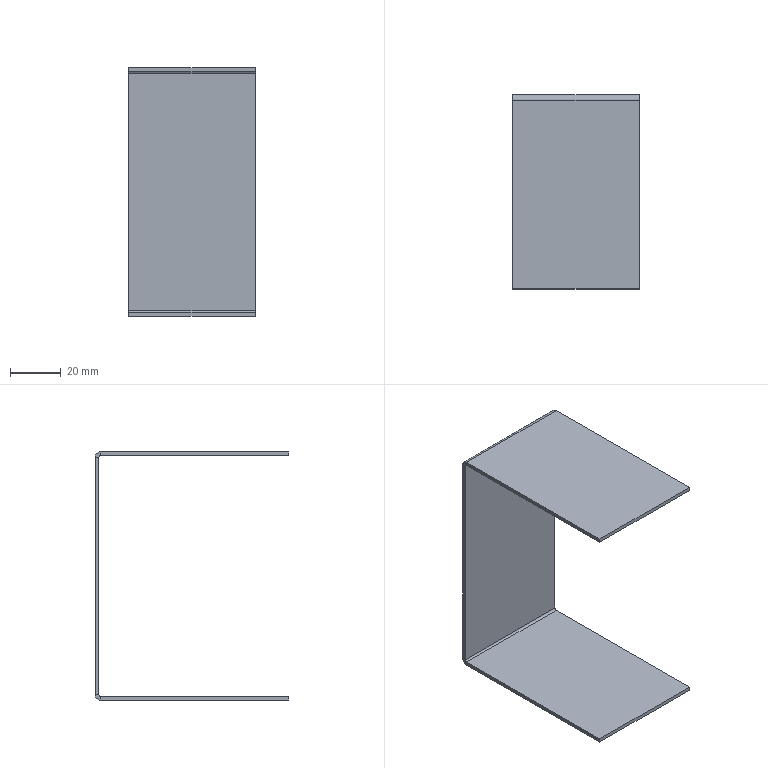Part | NX | 1 solid | 22 faces | box 50 x 76.5 x 98 mm | volume 18504 mm3 | plane 18 | cylinder 4 | commonest cylinder face diameters 1.473 x2 4.473 x2
STEP:
#1=CARTESIAN_POINT('',(-25.,-1.5,-46.763));
#2=VERTEX_POINT('',#1);
#3=CARTESIAN_POINT('',(-25.,-1.5,46.763));
#4=VERTEX_POINT('',#3);
#5=CARTESIAN_POINT('',(-25.,-1.5,47.5));
#6=DIRECTION('',(0.,0.,1.));
#7=VECTOR('',#6,1000.);
#8=LINE('',#5,#7);
#9=EDGE_CURVE('',#2,#4,#8,.T.);
#10=ORIENTED_EDGE('',*,*,#9,.F.);
#11=CARTESIAN_POINT('',(25.,-1.5,-46.763));
#12=VERTEX_POINT('',#11);
#13=CARTESIAN_POINT('',(25.,-1.5,-46.763));
#14=DIRECTION('',(1.,0.,0.));
#15=VECTOR('',#14,1000.);
#16=LINE('',#13,#15);
#17=EDGE_CURVE('',#12,#2,#16,.F.);
#18=ORIENTED_EDGE('',*,*,#17,.F.);
#19=CARTESIAN_POINT('',(25.,-1.5,46.763));
#20=VERTEX_POINT('',#19);
#21=CARTESIAN_POINT('',(25.,-1.5,47.5));
#22=DIRECTION('',(0.,0.,-1.));
#23=VECTOR('',#22,1000.);
#24=LINE('',#21,#23);
#25=EDGE_CURVE('',#20,#12,#24,.T.);
#26=ORIENTED_EDGE('',*,*,#25,.F.);
#27=CARTESIAN_POINT('',(-25.,-1.5,46.763));
#28=DIRECTION('',(-1.,0.,0.));
#29=VECTOR('',#28,1000.);
#30=LINE('',#27,#29);
#31=EDGE_CURVE('',#4,#20,#30,.F.);
#32=ORIENTED_EDGE('',*,*,#31,.F.);
#33=EDGE_LOOP('',(#10,#18,#26,#32));
#34=FACE_BOUND('',#33,.T.);
#35=CARTESIAN_POINT('',(0.,-1.5,0.));
#36=DIRECTION('',(0.,-1.,0.));
#37=DIRECTION('',(0.,0.,-1.));
#38=AXIS2_PLACEMENT_3D('',#35,#36,#37);
#39=PLANE('',#38);
#40=ADVANCED_FACE('',(#34),#39,.T.);
#41=CARTESIAN_POINT('',(25.,0.,-46.763));
#42=VERTEX_POINT('',#41);
#43=CARTESIAN_POINT('',(-25.,0.,-46.763));
#44=VERTEX_POINT('',#43);
#45=CARTESIAN_POINT('',(25.,0.,-46.763));
#46=DIRECTION('',(1.,0.,0.));
#47=VECTOR('',#46,1000.);
#48=LINE('',#45,#47);
#49=EDGE_CURVE('',#42,#44,#48,.F.);
#50=ORIENTED_EDGE('',*,*,#49,.T.);
#51=CARTESIAN_POINT('',(-25.,0.,46.763));
#52=VERTEX_POINT('',#51);
#53=CARTESIAN_POINT('',(-25.,0.,47.5));
#54=DIRECTION('',(0.,0.,1.));
#55=VECTOR('',#54,1000.);
#56=LINE('',#53,#55);
#57=EDGE_CURVE('',#44,#52,#56,.T.);
#58=ORIENTED_EDGE('',*,*,#57,.T.);
#59=CARTESIAN_POINT('',(25.,0.,46.763));
#60=VERTEX_POINT('',#59);
#61=CARTESIAN_POINT('',(-25.,0.,46.763));
#62=DIRECTION('',(-1.,0.,0.));
#63=VECTOR('',#62,1000.);
#64=LINE('',#61,#63);
#65=EDGE_CURVE('',#52,#60,#64,.F.);
#66=ORIENTED_EDGE('',*,*,#65,.T.);
#67=CARTESIAN_POINT('',(25.,0.,47.5));
#68=DIRECTION('',(0.,0.,-1.));
#69=VECTOR('',#68,1000.);
#70=LINE('',#67,#69);
#71=EDGE_CURVE('',#60,#42,#70,.T.);
#72=ORIENTED_EDGE('',*,*,#71,.T.);
#73=EDGE_LOOP('',(#50,#58,#66,#72));
#74=FACE_BOUND('',#73,.T.);
#75=CARTESIAN_POINT('',(0.,0.,0.));
#76=DIRECTION('',(0.,-1.,0.));
#77=DIRECTION('',(0.,0.,-1.));
#78=AXIS2_PLACEMENT_3D('',#75,#76,#77);
#79=PLANE('',#78);
#80=ADVANCED_FACE('',(#74),#79,.F.);
#81=ORIENTED_EDGE('',*,*,#25,.T.);
#82=CARTESIAN_POINT('',(25.,-1.5,-46.763));
#83=DIRECTION('',(0.,1.,0.));
#84=VECTOR('',#83,1000.);
#85=LINE('',#82,#84);
#86=EDGE_CURVE('',#12,#42,#85,.T.);
#87=ORIENTED_EDGE('',*,*,#86,.T.);
#88=ORIENTED_EDGE('',*,*,#71,.F.);
#89=CARTESIAN_POINT('',(25.,-1.5,46.763));
#90=DIRECTION('',(0.,1.,0.));
#91=VECTOR('',#90,1000.);
#92=LINE('',#89,#91);
#93=EDGE_CURVE('',#20,#60,#92,.T.);
#94=ORIENTED_EDGE('',*,*,#93,.F.);
#95=EDGE_LOOP('',(#81,#87,#88,#94));
#96=FACE_BOUND('',#95,.T.);
#97=CARTESIAN_POINT('',(25.,-1.5,47.5));
#98=DIRECTION('',(1.,0.,0.));
#99=DIRECTION('',(0.,0.,-1.));
#100=AXIS2_PLACEMENT_3D('',#97,#98,#99);
#101=PLANE('',#100);
#102=ADVANCED_FACE('',(#96),#101,.T.);
#103=CARTESIAN_POINT('',(-25.,-1.5,-46.763));
#104=DIRECTION('',(0.,1.,0.));
#105=VECTOR('',#104,1000.);
#106=LINE('',#103,#105);
#107=EDGE_CURVE('',#2,#44,#106,.T.);
#108=ORIENTED_EDGE('',*,*,#107,.F.);
#109=ORIENTED_EDGE('',*,*,#9,.T.);
#110=CARTESIAN_POINT('',(-25.,-1.5,46.763));
#111=DIRECTION('',(0.,1.,0.));
#112=VECTOR('',#111,1000.);
#113=LINE('',#110,#112);
#114=EDGE_CURVE('',#4,#52,#113,.T.);
#115=ORIENTED_EDGE('',*,*,#114,.T.);
#116=ORIENTED_EDGE('',*,*,#57,.F.);
#117=EDGE_LOOP('',(#108,#109,#115,#116));
#118=FACE_BOUND('',#117,.T.);
#119=CARTESIAN_POINT('',(-25.,-1.5,47.5));
#120=DIRECTION('',(-1.,0.,0.));
#121=DIRECTION('',(0.,0.,1.));
#122=AXIS2_PLACEMENT_3D('',#119,#120,#121);
#123=PLANE('',#122);
#124=ADVANCED_FACE('',(#118),#123,.T.);
#125=CARTESIAN_POINT('',(25.,-2.237,47.5));
#126=VERTEX_POINT('',#125);
#127=CARTESIAN_POINT('',(25.,-2.237,49.));
#128=VERTEX_POINT('',#127);
#129=CARTESIAN_POINT('',(25.,-2.237,47.5));
#130=DIRECTION('',(0.,0.,1.));
#131=VECTOR('',#130,1000.);
#132=LINE('',#129,#131);
#133=EDGE_CURVE('',#126,#128,#132,.T.);
#134=ORIENTED_EDGE('',*,*,#133,.F.);
#135=CARTESIAN_POINT('',(25.,-2.237,46.763));
#136=DIRECTION('',(-1.,0.,0.));
#137=DIRECTION('',(0.,0.,1.));
#138=AXIS2_PLACEMENT_3D('',#135,#136,#137);
#139=CIRCLE('',#138,0.7366);
#140=EDGE_CURVE('',#20,#126,#139,.F.);
#141=ORIENTED_EDGE('',*,*,#140,.F.);
#142=ORIENTED_EDGE('',*,*,#93,.T.);
#143=CARTESIAN_POINT('',(25.,-2.237,46.763));
#144=DIRECTION('',(-1.,0.,0.));
#145=DIRECTION('',(0.,0.,1.));
#146=AXIS2_PLACEMENT_3D('',#143,#144,#145);
#147=CIRCLE('',#146,2.237);
#148=EDGE_CURVE('',#60,#128,#147,.F.);
#149=ORIENTED_EDGE('',*,*,#148,.T.);
#150=EDGE_LOOP('',(#134,#141,#142,#149));
#151=FACE_BOUND('',#150,.T.);
#152=CARTESIAN_POINT('',(25.,-2.237,46.763));
#153=DIRECTION('',(1.,0.,0.));
#154=DIRECTION('',(0.,0.,-1.));
#155=AXIS2_PLACEMENT_3D('',#152,#153,#154);
#156=PLANE('',#155);
#157=ADVANCED_FACE('',(#151),#156,.T.);
#158=CARTESIAN_POINT('',(-25.,-2.237,47.5));
#159=VERTEX_POINT('',#158);
#160=CARTESIAN_POINT('',(-25.,-2.237,46.763));
#161=DIRECTION('',(-1.,0.,0.));
#162=DIRECTION('',(0.,0.,1.));
#163=AXIS2_PLACEMENT_3D('',#160,#161,#162);
#164=CIRCLE('',#163,0.7366);
#165=EDGE_CURVE('',#159,#4,#164,.T.);
#166=ORIENTED_EDGE('',*,*,#165,.F.);
#167=CARTESIAN_POINT('',(-25.,-2.237,49.));
#168=VERTEX_POINT('',#167);
#169=CARTESIAN_POINT('',(-25.,-2.237,47.5));
#170=DIRECTION('',(0.,0.,1.));
#171=VECTOR('',#170,1000.);
#172=LINE('',#169,#171);
#173=EDGE_CURVE('',#159,#168,#172,.T.);
#174=ORIENTED_EDGE('',*,*,#173,.T.);
#175=CARTESIAN_POINT('',(-25.,-2.237,46.763));
#176=DIRECTION('',(-1.,0.,0.));
#177=DIRECTION('',(0.,0.,1.));
#178=AXIS2_PLACEMENT_3D('',#175,#176,#177);
#179=CIRCLE('',#178,2.237);
#180=EDGE_CURVE('',#168,#52,#179,.T.);
#181=ORIENTED_EDGE('',*,*,#180,.T.);
#182=ORIENTED_EDGE('',*,*,#114,.F.);
#183=EDGE_LOOP('',(#166,#174,#181,#182));
#184=FACE_BOUND('',#183,.T.);
#185=CARTESIAN_POINT('',(-25.,-2.237,46.763));
#186=DIRECTION('',(1.,0.,0.));
#187=DIRECTION('',(0.,0.,-1.));
#188=AXIS2_PLACEMENT_3D('',#185,#186,#187);
#189=PLANE('',#188);
#190=ADVANCED_FACE('',(#184),#189,.F.);
#191=ORIENTED_EDGE('',*,*,#65,.F.);
#192=ORIENTED_EDGE('',*,*,#180,.F.);
#193=CARTESIAN_POINT('',(0.,-2.237,49.));
#194=DIRECTION('',(-1.,0.,0.));
#195=VECTOR('',#194,1000.);
#196=LINE('',#193,#195);
#197=EDGE_CURVE('',#128,#168,#196,.T.);
#198=ORIENTED_EDGE('',*,*,#197,.F.);
#199=ORIENTED_EDGE('',*,*,#148,.F.);
#200=EDGE_LOOP('',(#191,#192,#198,#199));
#201=FACE_BOUND('',#200,.T.);
#202=CARTESIAN_POINT('',(-25.,-2.237,46.763));
#203=DIRECTION('',(-1.,0.,0.));
#204=DIRECTION('',(0.,0.,1.));
#205=AXIS2_PLACEMENT_3D('',#202,#203,#204);
#206=CYLINDRICAL_SURFACE('',#205,2.237);
#207=ADVANCED_FACE('',(#201),#206,.T.);
#208=ORIENTED_EDGE('',*,*,#31,.T.);
#209=ORIENTED_EDGE('',*,*,#140,.T.);
#210=CARTESIAN_POINT('',(25.,-2.237,47.5));
#211=DIRECTION('',(-1.,0.,0.));
#212=VECTOR('',#211,1000.);
#213=LINE('',#210,#212);
#214=EDGE_CURVE('',#126,#159,#213,.T.);
#215=ORIENTED_EDGE('',*,*,#214,.T.);
#216=ORIENTED_EDGE('',*,*,#165,.T.);
#217=EDGE_LOOP('',(#208,#209,#215,#216));
#218=FACE_BOUND('',#217,.T.);
#219=CARTESIAN_POINT('',(-25.,-2.237,46.763));
#220=DIRECTION('',(-1.,0.,0.));
#221=DIRECTION('',(0.,0.,1.));
#222=AXIS2_PLACEMENT_3D('',#219,#220,#221);
#223=CYLINDRICAL_SURFACE('',#222,0.7366);
#224=ADVANCED_FACE('',(#218),#223,.F.);
#225=CARTESIAN_POINT('',(-25.,-76.5,49.));
#226=VERTEX_POINT('',#225);
#227=CARTESIAN_POINT('',(-25.,-1.5,49.));
#228=DIRECTION('',(0.,1.,0.));
#229=VECTOR('',#228,1000.);
#230=LINE('',#227,#229);
#231=EDGE_CURVE('',#226,#168,#230,.T.);
#232=ORIENTED_EDGE('',*,*,#231,.T.);
#233=ORIENTED_EDGE('',*,*,#173,.F.);
#234=CARTESIAN_POINT('',(-25.,-76.5,47.5));
#235=VERTEX_POINT('',#234);
#236=CARTESIAN_POINT('',(-25.,-1.5,47.5));
#237=DIRECTION('',(0.,1.,0.));
#238=VECTOR('',#237,1000.);
#239=LINE('',#236,#238);
#240=EDGE_CURVE('',#235,#159,#239,.T.);
#241=ORIENTED_EDGE('',*,*,#240,.F.);
#242=CARTESIAN_POINT('',(-25.,-76.5,49.));
#243=DIRECTION('',(0.,0.,-1.));
#244=VECTOR('',#243,1000.);
#245=LINE('',#242,#244);
#246=EDGE_CURVE('',#226,#235,#245,.T.);
#247=ORIENTED_EDGE('',*,*,#246,.F.);
#248=EDGE_LOOP('',(#232,#233,#241,#247));
#249=FACE_BOUND('',#248,.T.);
#250=CARTESIAN_POINT('',(-25.,-1.5,49.));
#251=DIRECTION('',(-1.,0.,0.));
#252=DIRECTION('',(0.,-1.,0.));
#253=AXIS2_PLACEMENT_3D('',#250,#251,#252);
#254=PLANE('',#253);
#255=ADVANCED_FACE('',(#249),#254,.T.);
#256=CARTESIAN_POINT('',(25.,-76.5,47.5));
#257=VERTEX_POINT('',#256);
#258=CARTESIAN_POINT('',(25.,-76.5,47.5));
#259=DIRECTION('',(0.,-1.,0.));
#260=VECTOR('',#259,1000.);
#261=LINE('',#258,#260);
#262=EDGE_CURVE('',#126,#257,#261,.T.);
#263=ORIENTED_EDGE('',*,*,#262,.F.);
#264=ORIENTED_EDGE('',*,*,#133,.T.);
#265=CARTESIAN_POINT('',(25.,-76.5,49.));
#266=VERTEX_POINT('',#265);
#267=CARTESIAN_POINT('',(25.,-76.5,49.));
#268=DIRECTION('',(0.,-1.,0.));
#269=VECTOR('',#268,1000.);
#270=LINE('',#267,#269);
#271=EDGE_CURVE('',#128,#266,#270,.T.);
#272=ORIENTED_EDGE('',*,*,#271,.T.);
#273=CARTESIAN_POINT('',(25.,-76.5,49.));
#274=DIRECTION('',(0.,0.,-1.));
#275=VECTOR('',#274,1000.);
#276=LINE('',#273,#275);
#277=EDGE_CURVE('',#266,#257,#276,.T.);
#278=ORIENTED_EDGE('',*,*,#277,.T.);
#279=EDGE_LOOP('',(#263,#264,#272,#278));
#280=FACE_BOUND('',#279,.T.);
#281=CARTESIAN_POINT('',(25.,-76.5,49.));
#282=DIRECTION('',(1.,0.,0.));
#283=DIRECTION('',(0.,1.,0.));
#284=AXIS2_PLACEMENT_3D('',#281,#282,#283);
#285=PLANE('',#284);
#286=ADVANCED_FACE('',(#280),#285,.T.);
#287=ORIENTED_EDGE('',*,*,#271,.F.);
#288=ORIENTED_EDGE('',*,*,#197,.T.);
#289=ORIENTED_EDGE('',*,*,#231,.F.);
#290=CARTESIAN_POINT('',(-25.,-76.5,49.));
#291=DIRECTION('',(-1.,0.,0.));
#292=VECTOR('',#291,1000.);
#293=LINE('',#290,#292);
#294=EDGE_CURVE('',#266,#226,#293,.T.);
#295=ORIENTED_EDGE('',*,*,#294,.F.);
#296=EDGE_LOOP('',(#287,#288,#289,#295));
#297=FACE_BOUND('',#296,.T.);
#298=CARTESIAN_POINT('',(0.,0.,49.));
#299=DIRECTION('',(0.,0.,1.));
#300=DIRECTION('',(0.,-1.,0.));
#301=AXIS2_PLACEMENT_3D('',#298,#299,#300);
#302=PLANE('',#301);
#303=ADVANCED_FACE('',(#297),#302,.T.);
#304=ORIENTED_EDGE('',*,*,#214,.F.);
#305=ORIENTED_EDGE('',*,*,#262,.T.);
#306=CARTESIAN_POINT('',(-25.,-76.5,47.5));
#307=DIRECTION('',(-1.,0.,0.));
#308=VECTOR('',#307,1000.);
#309=LINE('',#306,#308);
#310=EDGE_CURVE('',#257,#235,#309,.T.);
#311=ORIENTED_EDGE('',*,*,#310,.T.);
#312=ORIENTED_EDGE('',*,*,#240,.T.);
#313=EDGE_LOOP('',(#304,#305,#311,#312));
#314=FACE_BOUND('',#313,.T.);
#315=CARTESIAN_POINT('',(0.,0.,47.5));
#316=DIRECTION('',(0.,0.,1.));
#317=DIRECTION('',(0.,-1.,0.));
#318=AXIS2_PLACEMENT_3D('',#315,#316,#317);
#319=PLANE('',#318);
#320=ADVANCED_FACE('',(#314),#319,.F.);
#321=ORIENTED_EDGE('',*,*,#310,.F.);
#322=ORIENTED_EDGE('',*,*,#277,.F.);
#323=ORIENTED_EDGE('',*,*,#294,.T.);
#324=ORIENTED_EDGE('',*,*,#246,.T.);
#325=EDGE_LOOP('',(#321,#322,#323,#324));
#326=FACE_BOUND('',#325,.T.);
#327=CARTESIAN_POINT('',(-25.,-76.5,49.));
#328=DIRECTION('',(0.,-1.,0.));
#329=DIRECTION('',(0.,0.,-1.));
#330=AXIS2_PLACEMENT_3D('',#327,#328,#329);
#331=PLANE('',#330);
#332=ADVANCED_FACE('',(#326),#331,.T.);
#333=CARTESIAN_POINT('',(-25.,-2.237,-47.5));
#334=VERTEX_POINT('',#333);
#335=CARTESIAN_POINT('',(-25.,-2.237,-49.));
#336=VERTEX_POINT('',#335);
#337=CARTESIAN_POINT('',(-25.,-2.237,-47.5));
#338=DIRECTION('',(0.,0.,-1.));
#339=VECTOR('',#338,1000.);
#340=LINE('',#337,#339);
#341=EDGE_CURVE('',#334,#336,#340,.T.);
#342=ORIENTED_EDGE('',*,*,#341,.F.);
#343=CARTESIAN_POINT('',(-25.,-2.237,-46.763));
#344=DIRECTION('',(1.,0.,0.));
#345=DIRECTION('',(0.,0.,-1.));
#346=AXIS2_PLACEMENT_3D('',#343,#344,#345);
#347=CIRCLE('',#346,0.7366);
#348=EDGE_CURVE('',#2,#334,#347,.F.);
#349=ORIENTED_EDGE('',*,*,#348,.F.);
#350=ORIENTED_EDGE('',*,*,#107,.T.);
#351=CARTESIAN_POINT('',(-25.,-2.237,-46.763));
#352=DIRECTION('',(1.,0.,0.));
#353=DIRECTION('',(0.,0.,-1.));
#354=AXIS2_PLACEMENT_3D('',#351,#352,#353);
#355=CIRCLE('',#354,2.237);
#356=EDGE_CURVE('',#44,#336,#355,.F.);
#357=ORIENTED_EDGE('',*,*,#356,.T.);
#358=EDGE_LOOP('',(#342,#349,#350,#357));
#359=FACE_BOUND('',#358,.T.);
#360=CARTESIAN_POINT('',(-25.,-2.237,-46.763));
#361=DIRECTION('',(-1.,0.,0.));
#362=DIRECTION('',(0.,0.,1.));
#363=AXIS2_PLACEMENT_3D('',#360,#361,#362);
#364=PLANE('',#363);
#365=ADVANCED_FACE('',(#359),#364,.T.);
#366=CARTESIAN_POINT('',(25.,-2.237,-47.5));
#367=VERTEX_POINT('',#366);
#368=CARTESIAN_POINT('',(25.,-2.237,-46.763));
#369=DIRECTION('',(1.,0.,0.));
#370=DIRECTION('',(0.,0.,-1.));
#371=AXIS2_PLACEMENT_3D('',#368,#369,#370);
#372=CIRCLE('',#371,0.7366);
#373=EDGE_CURVE('',#367,#12,#372,.T.);
#374=ORIENTED_EDGE('',*,*,#373,.F.);
#375=CARTESIAN_POINT('',(25.,-2.237,-49.));
#376=VERTEX_POINT('',#375);
#377=CARTESIAN_POINT('',(25.,-2.237,-47.5));
#378=DIRECTION('',(0.,0.,-1.));
#379=VECTOR('',#378,1000.);
#380=LINE('',#377,#379);
#381=EDGE_CURVE('',#367,#376,#380,.T.);
#382=ORIENTED_EDGE('',*,*,#381,.T.);
#383=CARTESIAN_POINT('',(25.,-2.237,-46.763));
#384=DIRECTION('',(1.,0.,0.));
#385=DIRECTION('',(0.,0.,-1.));
#386=AXIS2_PLACEMENT_3D('',#383,#384,#385);
#387=CIRCLE('',#386,2.237);
#388=EDGE_CURVE('',#376,#42,#387,.T.);
#389=ORIENTED_EDGE('',*,*,#388,.T.);
#390=ORIENTED_EDGE('',*,*,#86,.F.);
#391=EDGE_LOOP('',(#374,#382,#389,#390));
#392=FACE_BOUND('',#391,.T.);
#393=CARTESIAN_POINT('',(25.,-2.237,-46.763));
#394=DIRECTION('',(-1.,0.,0.));
#395=DIRECTION('',(0.,0.,1.));
#396=AXIS2_PLACEMENT_3D('',#393,#394,#395);
#397=PLANE('',#396);
#398=ADVANCED_FACE('',(#392),#397,.F.);
#399=ORIENTED_EDGE('',*,*,#49,.F.);
#400=ORIENTED_EDGE('',*,*,#388,.F.);
#401=CARTESIAN_POINT('',(0.,-2.237,-49.));
#402=DIRECTION('',(-1.,0.,0.));
#403=VECTOR('',#402,1000.);
#404=LINE('',#401,#403);
#405=EDGE_CURVE('',#376,#336,#404,.T.);
#406=ORIENTED_EDGE('',*,*,#405,.T.);
#407=ORIENTED_EDGE('',*,*,#356,.F.);
#408=EDGE_LOOP('',(#399,#400,#406,#407));
#409=FACE_BOUND('',#408,.T.);
#410=CARTESIAN_POINT('',(25.,-2.237,-46.763));
#411=DIRECTION('',(1.,0.,0.));
#412=DIRECTION('',(0.,0.,-1.));
#413=AXIS2_PLACEMENT_3D('',#410,#411,#412);
#414=CYLINDRICAL_SURFACE('',#413,2.237);
#415=ADVANCED_FACE('',(#409),#414,.T.);
#416=ORIENTED_EDGE('',*,*,#17,.T.);
#417=ORIENTED_EDGE('',*,*,#348,.T.);
#418=CARTESIAN_POINT('',(-25.,-2.237,-47.5));
#419=DIRECTION('',(1.,0.,0.));
#420=VECTOR('',#419,1000.);
#421=LINE('',#418,#420);
#422=EDGE_CURVE('',#334,#367,#421,.T.);
#423=ORIENTED_EDGE('',*,*,#422,.T.);
#424=ORIENTED_EDGE('',*,*,#373,.T.);
#425=EDGE_LOOP('',(#416,#417,#423,#424));
#426=FACE_BOUND('',#425,.T.);
#427=CARTESIAN_POINT('',(25.,-2.237,-46.763));
#428=DIRECTION('',(1.,0.,0.));
#429=DIRECTION('',(0.,0.,-1.));
#430=AXIS2_PLACEMENT_3D('',#427,#428,#429);
#431=CYLINDRICAL_SURFACE('',#430,0.7366);
#432=ADVANCED_FACE('',(#426),#431,.F.);
#433=CARTESIAN_POINT('',(-25.,-76.5,-47.5));
#434=VERTEX_POINT('',#433);
#435=CARTESIAN_POINT('',(-25.,-1.5,-47.5));
#436=DIRECTION('',(0.,-1.,0.));
#437=VECTOR('',#436,1000.);
#438=LINE('',#435,#437);
#439=EDGE_CURVE('',#334,#434,#438,.T.);
#440=ORIENTED_EDGE('',*,*,#439,.F.);
#441=ORIENTED_EDGE('',*,*,#341,.T.);
#442=CARTESIAN_POINT('',(-25.,-76.5,-49.));
#443=VERTEX_POINT('',#442);
#444=CARTESIAN_POINT('',(-25.,-1.5,-49.));
#445=DIRECTION('',(0.,-1.,0.));
#446=VECTOR('',#445,1000.);
#447=LINE('',#444,#446);
#448=EDGE_CURVE('',#336,#443,#447,.T.);
#449=ORIENTED_EDGE('',*,*,#448,.T.);
#450=CARTESIAN_POINT('',(-25.,-76.5,-49.));
#451=DIRECTION('',(0.,0.,1.));
#452=VECTOR('',#451,1000.);
#453=LINE('',#450,#452);
#454=EDGE_CURVE('',#443,#434,#453,.T.);
#455=ORIENTED_EDGE('',*,*,#454,.T.);
#456=EDGE_LOOP('',(#440,#441,#449,#455));
#457=FACE_BOUND('',#456,.T.);
#458=CARTESIAN_POINT('',(-25.,-1.5,-49.));
#459=DIRECTION('',(-1.,0.,0.));
#460=DIRECTION('',(0.,-1.,0.));
#461=AXIS2_PLACEMENT_3D('',#458,#459,#460);
#462=PLANE('',#461);
#463=ADVANCED_FACE('',(#457),#462,.T.);
#464=CARTESIAN_POINT('',(25.,-76.5,-49.));
#465=VERTEX_POINT('',#464);
#466=CARTESIAN_POINT('',(25.,-76.5,-49.));
#467=DIRECTION('',(0.,1.,0.));
#468=VECTOR('',#467,1000.);
#469=LINE('',#466,#468);
#470=EDGE_CURVE('',#465,#376,#469,.T.);
#471=ORIENTED_EDGE('',*,*,#470,.T.);
#472=ORIENTED_EDGE('',*,*,#381,.F.);
#473=CARTESIAN_POINT('',(25.,-76.5,-47.5));
#474=VERTEX_POINT('',#473);
#475=CARTESIAN_POINT('',(25.,-76.5,-47.5));
#476=DIRECTION('',(0.,1.,0.));
#477=VECTOR('',#476,1000.);
#478=LINE('',#475,#477);
#479=EDGE_CURVE('',#474,#367,#478,.T.);
#480=ORIENTED_EDGE('',*,*,#479,.F.);
#481=CARTESIAN_POINT('',(25.,-76.5,-49.));
#482=DIRECTION('',(0.,0.,1.));
#483=VECTOR('',#482,1000.);
#484=LINE('',#481,#483);
#485=EDGE_CURVE('',#465,#474,#484,.T.);
#486=ORIENTED_EDGE('',*,*,#485,.F.);
#487=EDGE_LOOP('',(#471,#472,#480,#486));
#488=FACE_BOUND('',#487,.T.);
#489=CARTESIAN_POINT('',(25.,-76.5,-49.));
#490=DIRECTION('',(1.,0.,0.));
#491=DIRECTION('',(0.,1.,0.));
#492=AXIS2_PLACEMENT_3D('',#489,#490,#491);
#493=PLANE('',#492);
#494=ADVANCED_FACE('',(#488),#493,.T.);
#495=ORIENTED_EDGE('',*,*,#405,.F.);
#496=ORIENTED_EDGE('',*,*,#470,.F.);
#497=CARTESIAN_POINT('',(-25.,-76.5,-49.));
#498=DIRECTION('',(1.,0.,0.));
#499=VECTOR('',#498,1000.);
#500=LINE('',#497,#499);
#501=EDGE_CURVE('',#443,#465,#500,.T.);
#502=ORIENTED_EDGE('',*,*,#501,.F.);
#503=ORIENTED_EDGE('',*,*,#448,.F.);
#504=EDGE_LOOP('',(#495,#496,#502,#503));
#505=FACE_BOUND('',#504,.T.);
#506=CARTESIAN_POINT('',(0.,0.,-49.));
#507=DIRECTION('',(0.,0.,1.));
#508=DIRECTION('',(0.,-1.,0.));
#509=AXIS2_PLACEMENT_3D('',#506,#507,#508);
#510=PLANE('',#509);
#511=ADVANCED_FACE('',(#505),#510,.F.);
#512=ORIENTED_EDGE('',*,*,#479,.T.);
#513=ORIENTED_EDGE('',*,*,#422,.F.);
#514=ORIENTED_EDGE('',*,*,#439,.T.);
#515=CARTESIAN_POINT('',(-25.,-76.5,-47.5));
#516=DIRECTION('',(1.,0.,0.));
#517=VECTOR('',#516,1000.);
#518=LINE('',#515,#517);
#519=EDGE_CURVE('',#434,#474,#518,.T.);
#520=ORIENTED_EDGE('',*,*,#519,.T.);
#521=EDGE_LOOP('',(#512,#513,#514,#520));
#522=FACE_BOUND('',#521,.T.);
#523=CARTESIAN_POINT('',(0.,0.,-47.5));
#524=DIRECTION('',(0.,0.,1.));
#525=DIRECTION('',(0.,-1.,0.));
#526=AXIS2_PLACEMENT_3D('',#523,#524,#525);
#527=PLANE('',#526);
#528=ADVANCED_FACE('',(#522),#527,.T.);
#529=ORIENTED_EDGE('',*,*,#519,.F.);
#530=ORIENTED_EDGE('',*,*,#454,.F.);
#531=ORIENTED_EDGE('',*,*,#501,.T.);
#532=ORIENTED_EDGE('',*,*,#485,.T.);
#533=EDGE_LOOP('',(#529,#530,#531,#532));
#534=FACE_BOUND('',#533,.T.);
#535=CARTESIAN_POINT('',(-25.,-76.5,-49.));
#536=DIRECTION('',(0.,-1.,0.));
#537=DIRECTION('',(0.,0.,-1.));
#538=AXIS2_PLACEMENT_3D('',#535,#536,#537);
#539=PLANE('',#538);
#540=ADVANCED_FACE('',(#534),#539,.T.);
#541=CLOSED_SHELL('',(#40,#80,#102,#124,#157,#190,#207,#224,#255,#286,#303,#320,#332,#365,#398,#415,#432,#463,#494,#511,#528,#540));
#542=MANIFOLD_SOLID_BREP('',#541);
#543=(LENGTH_UNIT()NAMED_UNIT(*)SI_UNIT(.MILLI.,.METRE.));
#544=UNCERTAINTY_MEASURE_WITH_UNIT(LENGTH_MEASURE(0.00001),#543,'','');
#545=(NAMED_UNIT(*)PLANE_ANGLE_UNIT()SI_UNIT($,.RADIAN.));
#546=(NAMED_UNIT(*)SI_UNIT($,.STERADIAN.)SOLID_ANGLE_UNIT());
#547=(GEOMETRIC_REPRESENTATION_CONTEXT(3)GLOBAL_UNCERTAINTY_ASSIGNED_CONTEXT((#544))GLOBAL_UNIT_ASSIGNED_CONTEXT((#543,#545,#546))REPRESENTATION_CONTEXT('',''));
#548=ADVANCED_BREP_SHAPE_REPRESENTATION('',(#542),#547);